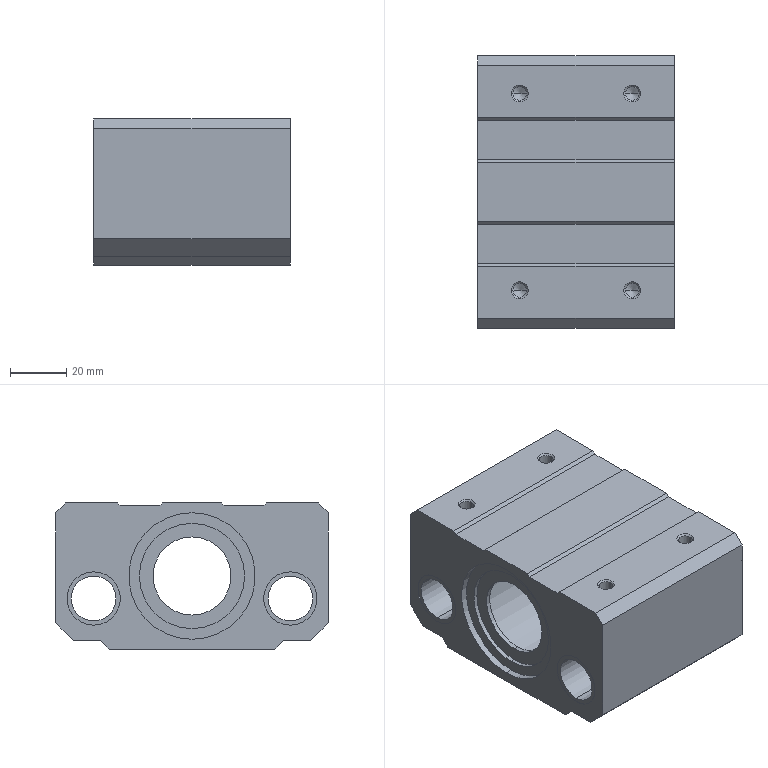Part | STEP file | _RMT-25X350-S(0)_body | 1 solid | 104 faces | box 70 x 97 x 52 mm | volume 215787 mm3 | cylinder 42 | plane 36 | cone 26 | commonest cylinder face diameters 4.917 x8 19 x8 4 x4 4.6 x4 16 x4 37.5 x4